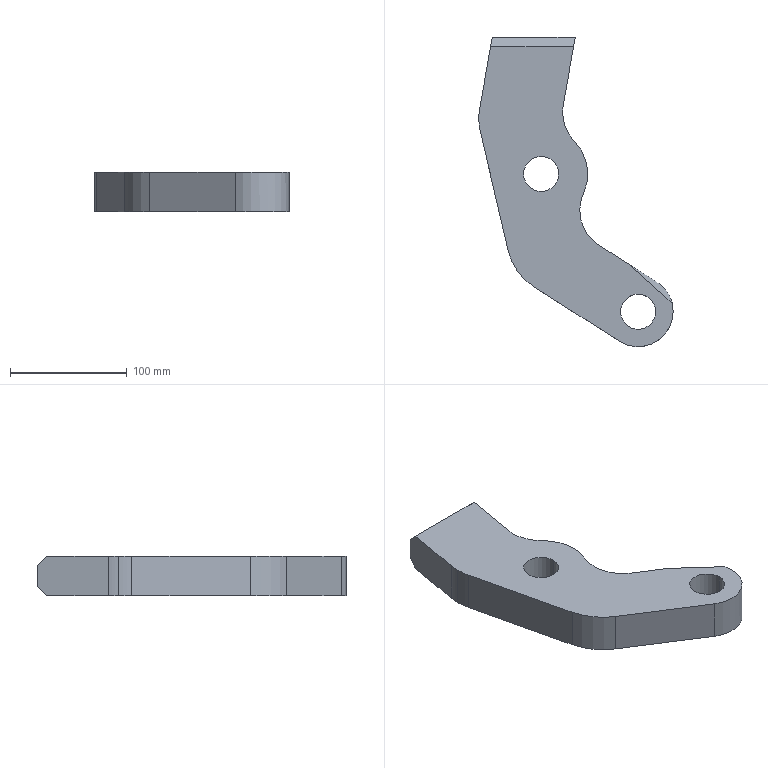Part | SolidWorks | features Fillet 2, ICE 2, Chamfer 1, Extrusion 1 | 1 solid | 24 faces | box 166.468 x 265 x 34 mm | volume 645452 mm3 | cylinder 13 | plane 11 | commonest cylinder face diameters 30 x4 70 x4 100 x3 60 x1 80 x1
STEP:
#1=CARTESIAN_POINT('',(-136.468,165.588,34.));
#2=VERTEX_POINT('',#1);
#3=CARTESIAN_POINT('',(-135.158,154.218,34.));
#4=VERTEX_POINT('',#3);
#5=CARTESIAN_POINT('',(-86.468,165.588,34.));
#6=DIRECTION('',(0.,0.,1.));
#7=DIRECTION('',(1.,0.,0.));
#8=AXIS2_PLACEMENT_3D('',#5,#6,#7);
#9=CIRCLE('',#8,50.);
#10=EDGE_CURVE('',#2,#4,#9,.T.);
#11=ORIENTED_EDGE('',*,*,#10,.F.);
#12=CARTESIAN_POINT('',(-136.468,165.588,0.));
#13=VERTEX_POINT('',#12);
#14=CARTESIAN_POINT('',(-136.468,165.588,34.));
#15=DIRECTION('',(0.,0.,-1.));
#16=VECTOR('',#15,1000.);
#17=LINE('',#14,#16);
#18=EDGE_CURVE('',#2,#13,#17,.T.);
#19=ORIENTED_EDGE('',*,*,#18,.T.);
#20=CARTESIAN_POINT('',(-135.158,154.218,0.));
#21=VERTEX_POINT('',#20);
#22=CARTESIAN_POINT('',(-86.468,165.588,0.));
#23=DIRECTION('',(0.,0.,-1.));
#24=DIRECTION('',(1.,0.,0.));
#25=AXIS2_PLACEMENT_3D('',#22,#23,#24);
#26=CIRCLE('',#25,50.);
#27=EDGE_CURVE('',#21,#13,#26,.T.);
#28=ORIENTED_EDGE('',*,*,#27,.F.);
#29=CARTESIAN_POINT('',(-135.158,154.218,34.));
#30=DIRECTION('',(0.,0.,-1.));
#31=VECTOR('',#30,1000.);
#32=LINE('',#29,#31);
#33=EDGE_CURVE('',#4,#21,#32,.T.);
#34=ORIENTED_EDGE('',*,*,#33,.F.);
#35=EDGE_LOOP('',(#11,#19,#28,#34));
#36=FACE_OUTER_BOUND('',#35,.T.);
#37=CARTESIAN_POINT('',(-86.468,165.588,34.));
#38=DIRECTION('',(0.,0.,-1.));
#39=DIRECTION('',(-1.,0.,0.));
#40=AXIS2_PLACEMENT_3D('',#37,#38,#39);
#41=CYLINDRICAL_SURFACE('',#40,50.);
#42=ADVANCED_FACE('',(#36),#41,.T.);
#43=CARTESIAN_POINT('',(-64.722,170.676,34.));
#44=VERTEX_POINT('',#43);
#45=CARTESIAN_POINT('',(-64.19,176.753,34.));
#46=VERTEX_POINT('',#45);
#47=CARTESIAN_POINT('',(-29.722,170.676,34.));
#48=DIRECTION('',(0.,0.,-1.));
#49=DIRECTION('',(1.,0.,0.));
#50=AXIS2_PLACEMENT_3D('',#47,#48,#49);
#51=CIRCLE('',#50,35.);
#52=EDGE_CURVE('',#44,#46,#51,.T.);
#53=ORIENTED_EDGE('',*,*,#52,.F.);
#54=CARTESIAN_POINT('',(-64.722,170.676,0.));
#55=VERTEX_POINT('',#54);
#56=CARTESIAN_POINT('',(-64.722,170.676,34.));
#57=DIRECTION('',(0.,0.,-1.));
#58=VECTOR('',#57,1000.);
#59=LINE('',#56,#58);
#60=EDGE_CURVE('',#44,#55,#59,.T.);
#61=ORIENTED_EDGE('',*,*,#60,.T.);
#62=CARTESIAN_POINT('',(-64.19,176.753,0.));
#63=VERTEX_POINT('',#62);
#64=CARTESIAN_POINT('',(-29.722,170.676,0.));
#65=DIRECTION('',(0.,0.,1.));
#66=DIRECTION('',(1.,0.,0.));
#67=AXIS2_PLACEMENT_3D('',#64,#65,#66);
#68=CIRCLE('',#67,35.);
#69=EDGE_CURVE('',#63,#55,#68,.T.);
#70=ORIENTED_EDGE('',*,*,#69,.F.);
#71=CARTESIAN_POINT('',(-64.19,176.753,0.));
#72=DIRECTION('',(0.,0.,-1.));
#73=VECTOR('',#72,1000.);
#74=LINE('',#71,#73);
#75=EDGE_CURVE('',#46,#63,#74,.T.);
#76=ORIENTED_EDGE('',*,*,#75,.F.);
#77=EDGE_LOOP('',(#53,#61,#70,#76));
#78=FACE_OUTER_BOUND('',#77,.T.);
#79=CARTESIAN_POINT('',(-29.722,170.676,34.));
#80=DIRECTION('',(0.,0.,-1.));
#81=DIRECTION('',(-1.,0.,0.));
#82=AXIS2_PLACEMENT_3D('',#79,#80,#81);
#83=CYLINDRICAL_SURFACE('',#82,35.);
#84=ADVANCED_FACE('',(#78),#83,.F.);
#85=CARTESIAN_POINT('',(-49.979,86.645,34.));
#86=VERTEX_POINT('',#85);
#87=CARTESIAN_POINT('',(-46.773,101.277,34.));
#88=VERTEX_POINT('',#87);
#89=CARTESIAN_POINT('',(-14.979,86.645,34.));
#90=DIRECTION('',(0.,0.,-1.));
#91=DIRECTION('',(1.,0.,0.));
#92=AXIS2_PLACEMENT_3D('',#89,#90,#91);
#93=CIRCLE('',#92,35.);
#94=EDGE_CURVE('',#86,#88,#93,.T.);
#95=ORIENTED_EDGE('',*,*,#94,.F.);
#96=CARTESIAN_POINT('',(-49.979,86.645,0.));
#97=VERTEX_POINT('',#96);
#98=CARTESIAN_POINT('',(-49.979,86.645,34.));
#99=DIRECTION('',(0.,0.,-1.));
#100=VECTOR('',#99,1000.);
#101=LINE('',#98,#100);
#102=EDGE_CURVE('',#86,#97,#101,.T.);
#103=ORIENTED_EDGE('',*,*,#102,.T.);
#104=CARTESIAN_POINT('',(-46.773,101.277,0.));
#105=VERTEX_POINT('',#104);
#106=CARTESIAN_POINT('',(-14.979,86.645,0.));
#107=DIRECTION('',(0.,0.,1.));
#108=DIRECTION('',(1.,0.,0.));
#109=AXIS2_PLACEMENT_3D('',#106,#107,#108);
#110=CIRCLE('',#109,35.);
#111=EDGE_CURVE('',#105,#97,#110,.T.);
#112=ORIENTED_EDGE('',*,*,#111,.F.);
#113=CARTESIAN_POINT('',(-46.773,101.277,34.));
#114=DIRECTION('',(0.,0.,-1.));
#115=VECTOR('',#114,1000.);
#116=LINE('',#113,#115);
#117=EDGE_CURVE('',#88,#105,#116,.T.);
#118=ORIENTED_EDGE('',*,*,#117,.F.);
#119=EDGE_LOOP('',(#95,#103,#112,#118));
#120=FACE_OUTER_BOUND('',#119,.T.);
#121=CARTESIAN_POINT('',(-14.979,86.645,34.));
#122=DIRECTION('',(0.,0.,-1.));
#123=DIRECTION('',(-1.,0.,0.));
#124=AXIS2_PLACEMENT_3D('',#121,#122,#123);
#125=CYLINDRICAL_SURFACE('',#124,35.);
#126=ADVANCED_FACE('',(#120),#125,.F.);
#127=CARTESIAN_POINT('',(-68.121,118.,34.));
#128=VERTEX_POINT('',#127);
#129=CARTESIAN_POINT('',(-98.121,118.,34.));
#130=VERTEX_POINT('',#129);
#131=CARTESIAN_POINT('',(-83.121,118.,34.));
#132=DIRECTION('',(0.,0.,-1.));
#133=DIRECTION('',(-1.,0.,0.));
#134=AXIS2_PLACEMENT_3D('',#131,#132,#133);
#135=CIRCLE('',#134,15.);
#136=EDGE_CURVE('',#128,#130,#135,.T.);
#137=ORIENTED_EDGE('',*,*,#136,.F.);
#138=CARTESIAN_POINT('',(-68.121,118.,0.));
#139=VERTEX_POINT('',#138);
#140=CARTESIAN_POINT('',(-68.121,118.,34.));
#141=DIRECTION('',(0.,0.,-1.));
#142=VECTOR('',#141,1000.);
#143=LINE('',#140,#142);
#144=EDGE_CURVE('',#128,#139,#143,.T.);
#145=ORIENTED_EDGE('',*,*,#144,.T.);
#146=CARTESIAN_POINT('',(-98.121,118.,0.));
#147=VERTEX_POINT('',#146);
#148=CARTESIAN_POINT('',(-83.121,118.,0.));
#149=DIRECTION('',(0.,0.,-1.));
#150=DIRECTION('',(-1.,0.,0.));
#151=AXIS2_PLACEMENT_3D('',#148,#149,#150);
#152=CIRCLE('',#151,15.);
#153=EDGE_CURVE('',#139,#147,#152,.T.);
#154=ORIENTED_EDGE('',*,*,#153,.T.);
#155=CARTESIAN_POINT('',(-98.121,118.,34.));
#156=DIRECTION('',(0.,0.,-1.));
#157=VECTOR('',#156,1000.);
#158=LINE('',#155,#157);
#159=EDGE_CURVE('',#130,#147,#158,.T.);
#160=ORIENTED_EDGE('',*,*,#159,.F.);
#161=EDGE_LOOP('',(#137,#145,#154,#160));
#162=FACE_OUTER_BOUND('',#161,.T.);
#163=CARTESIAN_POINT('',(-83.121,118.,34.));
#164=DIRECTION('',(0.,0.,-1.));
#165=DIRECTION('',(-1.,0.,0.));
#166=AXIS2_PLACEMENT_3D('',#163,#164,#165);
#167=CYLINDRICAL_SURFACE('',#166,15.);
#168=ADVANCED_FACE('',(#162),#167,.F.);
#169=CARTESIAN_POINT('',(14.992,0.,34.));
#170=VERTEX_POINT('',#169);
#171=CARTESIAN_POINT('',(-15.008,0.,34.));
#172=VERTEX_POINT('',#171);
#173=CARTESIAN_POINT('',(-0.008419,0.,34.));
#174=DIRECTION('',(0.,0.,-1.));
#175=DIRECTION('',(-1.,0.,0.));
#176=AXIS2_PLACEMENT_3D('',#173,#174,#175);
#177=CIRCLE('',#176,15.);
#178=EDGE_CURVE('',#170,#172,#177,.T.);
#179=ORIENTED_EDGE('',*,*,#178,.F.);
#180=CARTESIAN_POINT('',(14.992,0.,0.));
#181=VERTEX_POINT('',#180);
#182=CARTESIAN_POINT('',(14.992,0.,34.));
#183=DIRECTION('',(0.,0.,-1.));
#184=VECTOR('',#183,1000.);
#185=LINE('',#182,#184);
#186=EDGE_CURVE('',#170,#181,#185,.T.);
#187=ORIENTED_EDGE('',*,*,#186,.T.);
#188=CARTESIAN_POINT('',(-15.008,0.,0.));
#189=VERTEX_POINT('',#188);
#190=CARTESIAN_POINT('',(-0.008419,0.,0.));
#191=DIRECTION('',(0.,0.,-1.));
#192=DIRECTION('',(-1.,0.,0.));
#193=AXIS2_PLACEMENT_3D('',#190,#191,#192);
#194=CIRCLE('',#193,15.);
#195=EDGE_CURVE('',#181,#189,#194,.T.);
#196=ORIENTED_EDGE('',*,*,#195,.T.);
#197=CARTESIAN_POINT('',(-15.008,0.,34.));
#198=DIRECTION('',(0.,0.,-1.));
#199=VECTOR('',#198,1000.);
#200=LINE('',#197,#199);
#201=EDGE_CURVE('',#172,#189,#200,.T.);
#202=ORIENTED_EDGE('',*,*,#201,.F.);
#203=EDGE_LOOP('',(#179,#187,#196,#202));
#204=FACE_OUTER_BOUND('',#203,.T.);
#205=CARTESIAN_POINT('',(-0.008419,0.,34.));
#206=DIRECTION('',(0.,0.,-1.));
#207=DIRECTION('',(-1.,0.,0.));
#208=AXIS2_PLACEMENT_3D('',#205,#206,#207);
#209=CYLINDRICAL_SURFACE('',#208,15.);
#210=ADVANCED_FACE('',(#204),#209,.F.);
#211=CARTESIAN_POINT('',(-55.331,227.,34.));
#212=VERTEX_POINT('',#211);
#213=CARTESIAN_POINT('',(-53.92,235.,34.));
#214=DIRECTION('',(0.1736,0.9848,0.));
#215=VECTOR('',#214,1000.);
#216=LINE('',#213,#215);
#217=EDGE_CURVE('',#46,#212,#216,.T.);
#218=ORIENTED_EDGE('',*,*,#217,.F.);
#219=ORIENTED_EDGE('',*,*,#75,.T.);
#220=CARTESIAN_POINT('',(-55.331,227.,0.));
#221=VERTEX_POINT('',#220);
#222=CARTESIAN_POINT('',(-53.92,235.,0.));
#223=DIRECTION('',(0.1736,0.9848,0.));
#224=VECTOR('',#223,1000.);
#225=LINE('',#222,#224);
#226=EDGE_CURVE('',#63,#221,#225,.T.);
#227=ORIENTED_EDGE('',*,*,#226,.T.);
#228=CARTESIAN_POINT('',(-53.92,235.,8.));
#229=VERTEX_POINT('',#228);
#230=CARTESIAN_POINT('',(-55.008,228.829,1.829));
#231=DIRECTION('',(0.1237,0.7017,0.7017));
#232=VECTOR('',#231,1000.);
#233=LINE('',#230,#232);
#234=EDGE_CURVE('',#221,#229,#233,.T.);
#235=ORIENTED_EDGE('',*,*,#234,.T.);
#236=CARTESIAN_POINT('',(-53.92,235.,26.));
#237=VERTEX_POINT('',#236);
#238=CARTESIAN_POINT('',(-53.92,235.,34.));
#239=DIRECTION('',(0.,0.,-1.));
#240=VECTOR('',#239,1000.);
#241=LINE('',#238,#240);
#242=EDGE_CURVE('',#237,#229,#241,.T.);
#243=ORIENTED_EDGE('',*,*,#242,.F.);
#244=CARTESIAN_POINT('',(-55.756,224.588,36.412));
#245=DIRECTION('',(-0.1237,-0.7017,0.7017));
#246=VECTOR('',#245,1000.);
#247=LINE('',#244,#246);
#248=EDGE_CURVE('',#237,#212,#247,.T.);
#249=ORIENTED_EDGE('',*,*,#248,.T.);
#250=EDGE_LOOP('',(#218,#219,#227,#235,#243,#249));
#251=FACE_OUTER_BOUND('',#250,.T.);
#252=CARTESIAN_POINT('',(-53.92,235.,34.));
#253=DIRECTION('',(-0.9848,0.1736,0.));
#254=DIRECTION('',(-0.1736,-0.9848,0.));
#255=AXIS2_PLACEMENT_3D('',#252,#253,#254);
#256=PLANE('',#255);
#257=ADVANCED_FACE('',(#251),#256,.F.);
#258=ORIENTED_EDGE('',*,*,#242,.T.);
#259=CARTESIAN_POINT('',(-125.,235.,8.));
#260=VERTEX_POINT('',#259);
#261=CARTESIAN_POINT('',(-125.,235.,8.));
#262=DIRECTION('',(-1.,0.,0.));
#263=VECTOR('',#262,1000.);
#264=LINE('',#261,#263);
#265=EDGE_CURVE('',#229,#260,#264,.T.);
#266=ORIENTED_EDGE('',*,*,#265,.T.);
#267=CARTESIAN_POINT('',(-125.,235.,26.));
#268=VERTEX_POINT('',#267);
#269=CARTESIAN_POINT('',(-125.,235.,34.));
#270=DIRECTION('',(0.,0.,-1.));
#271=VECTOR('',#270,1000.);
#272=LINE('',#269,#271);
#273=EDGE_CURVE('',#268,#260,#272,.T.);
#274=ORIENTED_EDGE('',*,*,#273,.F.);
#275=CARTESIAN_POINT('',(-53.92,235.,26.));
#276=DIRECTION('',(1.,0.,0.));
#277=VECTOR('',#276,1000.);
#278=LINE('',#275,#277);
#279=EDGE_CURVE('',#268,#237,#278,.T.);
#280=ORIENTED_EDGE('',*,*,#279,.T.);
#281=EDGE_LOOP('',(#258,#266,#274,#280));
#282=FACE_OUTER_BOUND('',#281,.T.);
#283=CARTESIAN_POINT('',(-125.,235.,34.));
#284=DIRECTION('',(0.,-1.,0.));
#285=DIRECTION('',(0.,0.,-1.));
#286=AXIS2_PLACEMENT_3D('',#283,#284,#285);
#287=PLANE('',#286);
#288=ADVANCED_FACE('',(#282),#287,.F.);
#289=CARTESIAN_POINT('',(-126.411,227.,0.));
#290=VERTEX_POINT('',#289);
#291=CARTESIAN_POINT('',(-135.708,174.271,0.));
#292=VERTEX_POINT('',#291);
#293=CARTESIAN_POINT('',(-125.,235.,0.));
#294=DIRECTION('',(-0.1736,-0.9848,0.));
#295=VECTOR('',#294,1000.);
#296=LINE('',#293,#295);
#297=EDGE_CURVE('',#290,#292,#296,.T.);
#298=ORIENTED_EDGE('',*,*,#297,.T.);
#299=CARTESIAN_POINT('',(-135.708,174.271,34.));
#300=VERTEX_POINT('',#299);
#301=CARTESIAN_POINT('',(-135.708,174.271,34.));
#302=DIRECTION('',(0.,0.,1.));
#303=VECTOR('',#302,1000.);
#304=LINE('',#301,#303);
#305=EDGE_CURVE('',#292,#300,#304,.T.);
#306=ORIENTED_EDGE('',*,*,#305,.T.);
#307=CARTESIAN_POINT('',(-126.411,227.,34.));
#308=VERTEX_POINT('',#307);
#309=CARTESIAN_POINT('',(-125.,235.,34.));
#310=DIRECTION('',(-0.1736,-0.9848,0.));
#311=VECTOR('',#310,1000.);
#312=LINE('',#309,#311);
#313=EDGE_CURVE('',#308,#300,#312,.T.);
#314=ORIENTED_EDGE('',*,*,#313,.F.);
#315=CARTESIAN_POINT('',(-125.748,230.759,30.241));
#316=DIRECTION('',(0.1237,0.7017,-0.7017));
#317=VECTOR('',#316,1000.);
#318=LINE('',#315,#317);
#319=EDGE_CURVE('',#308,#268,#318,.T.);
#320=ORIENTED_EDGE('',*,*,#319,.T.);
#321=ORIENTED_EDGE('',*,*,#273,.T.);
#322=CARTESIAN_POINT('',(-125.,235.,8.));
#323=DIRECTION('',(-0.1237,-0.7017,-0.7017));
#324=VECTOR('',#323,1000.);
#325=LINE('',#322,#324);
#326=EDGE_CURVE('',#260,#290,#325,.T.);
#327=ORIENTED_EDGE('',*,*,#326,.T.);
#328=EDGE_LOOP('',(#298,#306,#314,#320,#321,#327));
#329=FACE_OUTER_BOUND('',#328,.T.);
#330=CARTESIAN_POINT('',(-125.,235.,34.));
#331=DIRECTION('',(0.9848,-0.1736,0.));
#332=DIRECTION('',(0.1736,0.9848,0.));
#333=AXIS2_PLACEMENT_3D('',#330,#331,#332);
#334=PLANE('',#333);
#335=ADVANCED_FACE('',(#329),#334,.F.);
#336=CARTESIAN_POINT('',(-111.36,52.316,0.));
#337=VERTEX_POINT('',#336);
#338=CARTESIAN_POINT('',(-137.486,164.188,0.));
#339=DIRECTION('',(0.2274,-0.9738,0.));
#340=VECTOR('',#339,1000.);
#341=LINE('',#338,#340);
#342=EDGE_CURVE('',#21,#337,#341,.T.);
#343=ORIENTED_EDGE('',*,*,#342,.T.);
#344=CARTESIAN_POINT('',(-111.36,52.316,34.));
#345=VERTEX_POINT('',#344);
#346=CARTESIAN_POINT('',(-111.36,52.316,34.));
#347=DIRECTION('',(0.,0.,1.));
#348=VECTOR('',#347,1000.);
#349=LINE('',#346,#348);
#350=EDGE_CURVE('',#337,#345,#349,.T.);
#351=ORIENTED_EDGE('',*,*,#350,.T.);
#352=CARTESIAN_POINT('',(-137.486,164.188,34.));
#353=DIRECTION('',(0.2274,-0.9738,0.));
#354=VECTOR('',#353,1000.);
#355=LINE('',#352,#354);
#356=EDGE_CURVE('',#4,#345,#355,.T.);
#357=ORIENTED_EDGE('',*,*,#356,.F.);
#358=ORIENTED_EDGE('',*,*,#33,.T.);
#359=EDGE_LOOP('',(#343,#351,#357,#358));
#360=FACE_OUTER_BOUND('',#359,.T.);
#361=CARTESIAN_POINT('',(-137.486,164.188,34.));
#362=DIRECTION('',(0.9738,0.2274,0.));
#363=DIRECTION('',(-0.2274,0.9738,0.));
#364=AXIS2_PLACEMENT_3D('',#361,#362,#363);
#365=PLANE('',#364);
#366=ADVANCED_FACE('',(#360),#365,.F.);
#367=CARTESIAN_POINT('',(-89.555,21.529,34.));
#368=VERTEX_POINT('',#367);
#369=CARTESIAN_POINT('',(-16.131,-25.294,34.));
#370=VERTEX_POINT('',#369);
#371=CARTESIAN_POINT('',(-106.728,32.481,34.));
#372=DIRECTION('',(0.8431,-0.5377,0.));
#373=VECTOR('',#372,1000.);
#374=LINE('',#371,#373);
#375=EDGE_CURVE('',#368,#370,#374,.T.);
#376=ORIENTED_EDGE('',*,*,#375,.F.);
#377=CARTESIAN_POINT('',(-89.555,21.529,0.));
#378=VERTEX_POINT('',#377);
#379=CARTESIAN_POINT('',(-89.555,21.529,34.));
#380=DIRECTION('',(0.,0.,-1.));
#381=VECTOR('',#380,1000.);
#382=LINE('',#379,#381);
#383=EDGE_CURVE('',#368,#378,#382,.T.);
#384=ORIENTED_EDGE('',*,*,#383,.T.);
#385=CARTESIAN_POINT('',(-16.131,-25.294,0.));
#386=VERTEX_POINT('',#385);
#387=CARTESIAN_POINT('',(-106.728,32.481,0.));
#388=DIRECTION('',(0.8431,-0.5377,0.));
#389=VECTOR('',#388,1000.);
#390=LINE('',#387,#389);
#391=EDGE_CURVE('',#378,#386,#390,.T.);
#392=ORIENTED_EDGE('',*,*,#391,.T.);
#393=CARTESIAN_POINT('',(-16.131,-25.294,34.));
#394=DIRECTION('',(0.,0.,-1.));
#395=VECTOR('',#394,1000.);
#396=LINE('',#393,#395);
#397=EDGE_CURVE('',#370,#386,#396,.T.);
#398=ORIENTED_EDGE('',*,*,#397,.F.);
#399=EDGE_LOOP('',(#376,#384,#392,#398));
#400=FACE_OUTER_BOUND('',#399,.T.);
#401=CARTESIAN_POINT('',(-106.728,32.481,34.));
#402=DIRECTION('',(0.5377,0.8431,0.));
#403=DIRECTION('',(-0.8431,0.5377,0.));
#404=AXIS2_PLACEMENT_3D('',#401,#402,#403);
#405=PLANE('',#404);
#406=ADVANCED_FACE('',(#400),#405,.F.);
#407=CARTESIAN_POINT('',(16.131,25.294,22.982));
#408=VERTEX_POINT('',#407);
#409=CARTESIAN_POINT('',(29.052,7.482,34.));
#410=VERTEX_POINT('',#409);
#411=CARTESIAN_POINT('',(16.131,25.294,22.982));
#412=CARTESIAN_POINT('',(22.616,21.158,19.943));
#413=CARTESIAN_POINT('',(27.133,14.932,23.795));
#414=CARTESIAN_POINT('',(29.052,7.482,34.));
#415=(BOUNDED_CURVE()B_SPLINE_CURVE(3,(#411,#412,#413,#414),.UNSPECIFIED.,.F.,.F.)B_SPLINE_CURVE_WITH_KNOTS((4,4),(6.118,6.869),.UNSPECIFIED.)CURVE()GEOMETRIC_REPRESENTATION_ITEM()RATIONAL_B_SPLINE_CURVE((1.,0.9535,0.9535,1.))REPRESENTATION_ITEM(''));
#416=EDGE_CURVE('',#408,#410,#415,.T.);
#417=ORIENTED_EDGE('',*,*,#416,.T.);
#418=CARTESIAN_POINT('',(0.,0.,34.));
#419=DIRECTION('',(0.,0.,1.));
#420=DIRECTION('',(1.,0.,0.));
#421=AXIS2_PLACEMENT_3D('',#418,#419,#420);
#422=CIRCLE('',#421,30.);
#423=EDGE_CURVE('',#370,#410,#422,.T.);
#424=ORIENTED_EDGE('',*,*,#423,.F.);
#425=ORIENTED_EDGE('',*,*,#397,.T.);
#426=CARTESIAN_POINT('',(16.131,25.294,0.));
#427=VERTEX_POINT('',#426);
#428=CARTESIAN_POINT('',(0.,0.,0.));
#429=DIRECTION('',(0.,0.,1.));
#430=DIRECTION('',(1.,0.,0.));
#431=AXIS2_PLACEMENT_3D('',#428,#429,#430);
#432=CIRCLE('',#431,30.);
#433=EDGE_CURVE('',#386,#427,#432,.T.);
#434=ORIENTED_EDGE('',*,*,#433,.T.);
#435=CARTESIAN_POINT('',(16.131,25.294,34.));
#436=DIRECTION('',(0.,0.,-1.));
#437=VECTOR('',#436,1000.);
#438=LINE('',#435,#437);
#439=EDGE_CURVE('',#408,#427,#438,.T.);
#440=ORIENTED_EDGE('',*,*,#439,.F.);
#441=EDGE_LOOP('',(#417,#424,#425,#434,#440));
#442=FACE_OUTER_BOUND('',#441,.T.);
#443=CARTESIAN_POINT('',(0.,0.,34.));
#444=DIRECTION('',(0.,0.,-1.));
#445=DIRECTION('',(-1.,0.,0.));
#446=AXIS2_PLACEMENT_3D('',#443,#444,#445);
#447=CYLINDRICAL_SURFACE('',#446,30.);
#448=ADVANCED_FACE('',(#442),#447,.T.);
#449=CARTESIAN_POINT('',(-7.386,40.291,34.));
#450=VERTEX_POINT('',#449);
#451=CARTESIAN_POINT('',(-33.798,57.134,34.));
#452=VERTEX_POINT('',#451);
#453=CARTESIAN_POINT('',(-69.988,80.214,34.));
#454=DIRECTION('',(-0.8431,0.5377,0.));
#455=VECTOR('',#454,1000.);
#456=LINE('',#453,#455);
#457=EDGE_CURVE('',#450,#452,#456,.T.);
#458=ORIENTED_EDGE('',*,*,#457,.F.);
#459=CARTESIAN_POINT('',(-61.538,74.825,59.371));
#460=DIRECTION('',(0.7842,-0.5001,-0.3674));
#461=VECTOR('',#460,1000.);
#462=LINE('',#459,#461);
#463=EDGE_CURVE('',#450,#408,#462,.T.);
#464=ORIENTED_EDGE('',*,*,#463,.T.);
#465=ORIENTED_EDGE('',*,*,#439,.T.);
#466=CARTESIAN_POINT('',(-33.798,57.134,0.));
#467=VERTEX_POINT('',#466);
#468=CARTESIAN_POINT('',(-69.988,80.214,0.));
#469=DIRECTION('',(-0.8431,0.5377,0.));
#470=VECTOR('',#469,1000.);
#471=LINE('',#468,#470);
#472=EDGE_CURVE('',#427,#467,#471,.T.);
#473=ORIENTED_EDGE('',*,*,#472,.T.);
#474=CARTESIAN_POINT('',(-33.798,57.134,34.));
#475=DIRECTION('',(0.,0.,1.));
#476=VECTOR('',#475,1000.);
#477=LINE('',#474,#476);
#478=EDGE_CURVE('',#467,#452,#477,.T.);
#479=ORIENTED_EDGE('',*,*,#478,.T.);
#480=EDGE_LOOP('',(#458,#464,#465,#473,#479));
#481=FACE_OUTER_BOUND('',#480,.T.);
#482=CARTESIAN_POINT('',(-69.988,80.214,34.));
#483=DIRECTION('',(-0.5377,-0.8431,0.));
#484=DIRECTION('',(0.8431,-0.5377,0.));
#485=AXIS2_PLACEMENT_3D('',#482,#483,#484);
#486=PLANE('',#485);
#487=ADVANCED_FACE('',(#481),#486,.F.);
#488=CARTESIAN_POINT('',(-54.636,146.094,34.));
#489=VERTEX_POINT('',#488);
#490=CARTESIAN_POINT('',(-83.11,118.,34.));
#491=DIRECTION('',(0.,0.,1.));
#492=DIRECTION('',(1.,0.,0.));
#493=AXIS2_PLACEMENT_3D('',#490,#491,#492);
#494=CIRCLE('',#493,40.);
#495=EDGE_CURVE('',#88,#489,#494,.T.);
#496=ORIENTED_EDGE('',*,*,#495,.F.);
#497=ORIENTED_EDGE('',*,*,#117,.T.);
#498=CARTESIAN_POINT('',(-54.636,146.094,0.));
#499=VERTEX_POINT('',#498);
#500=CARTESIAN_POINT('',(-83.11,118.,0.));
#501=DIRECTION('',(0.,0.,1.));
#502=DIRECTION('',(1.,0.,0.));
#503=AXIS2_PLACEMENT_3D('',#500,#501,#502);
#504=CIRCLE('',#503,40.);
#505=EDGE_CURVE('',#105,#499,#504,.T.);
#506=ORIENTED_EDGE('',*,*,#505,.T.);
#507=CARTESIAN_POINT('',(-54.636,146.094,34.));
#508=DIRECTION('',(0.,0.,1.));
#509=VECTOR('',#508,1000.);
#510=LINE('',#507,#509);
#511=EDGE_CURVE('',#499,#489,#510,.T.);
#512=ORIENTED_EDGE('',*,*,#511,.T.);
#513=EDGE_LOOP('',(#496,#497,#506,#512));
#514=FACE_OUTER_BOUND('',#513,.T.);
#515=CARTESIAN_POINT('',(-83.11,118.,34.));
#516=DIRECTION('',(0.,0.,-1.));
#517=DIRECTION('',(-1.,0.,0.));
#518=AXIS2_PLACEMENT_3D('',#515,#516,#517);
#519=CYLINDRICAL_SURFACE('',#518,40.);
#520=ADVANCED_FACE('',(#514),#519,.T.);
#521=CARTESIAN_POINT('',(-175.495,191.658,34.));
#522=DIRECTION('',(0.7431,-0.6691,0.));
#523=VECTOR('',#522,1000.);
#524=LINE('',#521,#523);
#525=EDGE_CURVE('',#450,#410,#524,.T.);
#526=ORIENTED_EDGE('',*,*,#525,.F.);
#527=ORIENTED_EDGE('',*,*,#457,.T.);
#528=CARTESIAN_POINT('',(-14.979,86.645,34.));
#529=DIRECTION('',(0.,0.,-1.));
#530=DIRECTION('',(1.,0.,0.));
#531=AXIS2_PLACEMENT_3D('',#528,#529,#530);
#532=CIRCLE('',#531,35.);
#533=EDGE_CURVE('',#452,#86,#532,.T.);
#534=ORIENTED_EDGE('',*,*,#533,.T.);
#535=ORIENTED_EDGE('',*,*,#94,.T.);
#536=ORIENTED_EDGE('',*,*,#495,.T.);
#537=CARTESIAN_POINT('',(-29.722,170.676,34.));
#538=DIRECTION('',(0.,0.,-1.));
#539=DIRECTION('',(1.,0.,0.));
#540=AXIS2_PLACEMENT_3D('',#537,#538,#539);
#541=CIRCLE('',#540,35.);
#542=EDGE_CURVE('',#489,#44,#541,.T.);
#543=ORIENTED_EDGE('',*,*,#542,.T.);
#544=ORIENTED_EDGE('',*,*,#52,.T.);
#545=ORIENTED_EDGE('',*,*,#217,.T.);
#546=CARTESIAN_POINT('',(-125.,227.,34.));
#547=DIRECTION('',(-1.,0.,0.));
#548=VECTOR('',#547,1000.);
#549=LINE('',#546,#548);
#550=EDGE_CURVE('',#212,#308,#549,.T.);
#551=ORIENTED_EDGE('',*,*,#550,.T.);
#552=ORIENTED_EDGE('',*,*,#313,.T.);
#553=CARTESIAN_POINT('',(-86.468,165.588,34.));
#554=DIRECTION('',(0.,0.,1.));
#555=DIRECTION('',(1.,0.,0.));
#556=AXIS2_PLACEMENT_3D('',#553,#554,#555);
#557=CIRCLE('',#556,50.);
#558=EDGE_CURVE('',#300,#2,#557,.T.);
#559=ORIENTED_EDGE('',*,*,#558,.T.);
#560=ORIENTED_EDGE('',*,*,#10,.T.);
#561=ORIENTED_EDGE('',*,*,#356,.T.);
#562=CARTESIAN_POINT('',(-62.67,63.686,34.));
#563=DIRECTION('',(0.,0.,1.));
#564=DIRECTION('',(1.,0.,0.));
#565=AXIS2_PLACEMENT_3D('',#562,#563,#564);
#566=CIRCLE('',#565,50.);
#567=EDGE_CURVE('',#345,#368,#566,.T.);
#568=ORIENTED_EDGE('',*,*,#567,.T.);
#569=ORIENTED_EDGE('',*,*,#375,.T.);
#570=ORIENTED_EDGE('',*,*,#423,.T.);
#571=EDGE_LOOP('',(#526,#527,#534,#535,#536,#543,#544,#545,#551,#552,#559,#560,#561,#568,#569,#570));
#572=FACE_OUTER_BOUND('',#571,.T.);
#573=CARTESIAN_POINT('',(-83.121,118.,34.));
#574=DIRECTION('',(0.,0.,-1.));
#575=DIRECTION('',(-1.,0.,0.));
#576=AXIS2_PLACEMENT_3D('',#573,#574,#575);
#577=CIRCLE('',#576,15.);
#578=EDGE_CURVE('',#130,#128,#577,.T.);
#579=ORIENTED_EDGE('',*,*,#578,.T.);
#580=ORIENTED_EDGE('',*,*,#136,.T.);
#581=EDGE_LOOP('',(#579,#580));
#582=FACE_BOUND('',#581,.T.);
#583=CARTESIAN_POINT('',(-0.008419,0.,34.));
#584=DIRECTION('',(0.,0.,-1.));
#585=DIRECTION('',(-1.,0.,0.));
#586=AXIS2_PLACEMENT_3D('',#583,#584,#585);
#587=CIRCLE('',#586,15.);
#588=EDGE_CURVE('',#172,#170,#587,.T.);
#589=ORIENTED_EDGE('',*,*,#588,.T.);
#590=ORIENTED_EDGE('',*,*,#178,.T.);
#591=EDGE_LOOP('',(#589,#590));
#592=FACE_BOUND('',#591,.T.);
#593=CARTESIAN_POINT('',(-83.11,118.,34.));
#594=DIRECTION('',(0.,0.,1.));
#595=DIRECTION('',(1.,0.,0.));
#596=AXIS2_PLACEMENT_3D('',#593,#594,#595);
#597=PLANE('',#596);
#598=ADVANCED_FACE('',(#572,#582,#592),#597,.T.);
#599=CARTESIAN_POINT('',(-83.121,118.,0.));
#600=DIRECTION('',(0.,0.,-1.));
#601=DIRECTION('',(-1.,0.,0.));
#602=AXIS2_PLACEMENT_3D('',#599,#600,#601);
#603=CIRCLE('',#602,15.);
#604=EDGE_CURVE('',#147,#139,#603,.T.);
#605=ORIENTED_EDGE('',*,*,#604,.F.);
#606=ORIENTED_EDGE('',*,*,#153,.F.);
#607=EDGE_LOOP('',(#605,#606));
#608=FACE_BOUND('',#607,.T.);
#609=CARTESIAN_POINT('',(-0.008419,0.,0.));
#610=DIRECTION('',(0.,0.,-1.));
#611=DIRECTION('',(-1.,0.,0.));
#612=AXIS2_PLACEMENT_3D('',#609,#610,#611);
#613=CIRCLE('',#612,15.);
#614=EDGE_CURVE('',#189,#181,#613,.T.);
#615=ORIENTED_EDGE('',*,*,#614,.F.);
#616=ORIENTED_EDGE('',*,*,#195,.F.);
#617=EDGE_LOOP('',(#615,#616));
#618=FACE_BOUND('',#617,.T.);
#619=ORIENTED_EDGE('',*,*,#391,.F.);
#620=CARTESIAN_POINT('',(-62.67,63.686,0.));
#621=DIRECTION('',(0.,0.,-1.));
#622=DIRECTION('',(1.,0.,0.));
#623=AXIS2_PLACEMENT_3D('',#620,#621,#622);
#624=CIRCLE('',#623,50.);
#625=EDGE_CURVE('',#378,#337,#624,.T.);
#626=ORIENTED_EDGE('',*,*,#625,.T.);
#627=ORIENTED_EDGE('',*,*,#342,.F.);
#628=ORIENTED_EDGE('',*,*,#27,.T.);
#629=CARTESIAN_POINT('',(-86.468,165.588,0.));
#630=DIRECTION('',(0.,0.,-1.));
#631=DIRECTION('',(1.,0.,0.));
#632=AXIS2_PLACEMENT_3D('',#629,#630,#631);
#633=CIRCLE('',#632,50.);
#634=EDGE_CURVE('',#13,#292,#633,.T.);
#635=ORIENTED_EDGE('',*,*,#634,.T.);
#636=ORIENTED_EDGE('',*,*,#297,.F.);
#637=CARTESIAN_POINT('',(-83.11,227.,0.));
#638=DIRECTION('',(1.,0.,0.));
#639=VECTOR('',#638,1000.);
#640=LINE('',#637,#639);
#641=EDGE_CURVE('',#290,#221,#640,.T.);
#642=ORIENTED_EDGE('',*,*,#641,.T.);
#643=ORIENTED_EDGE('',*,*,#226,.F.);
#644=ORIENTED_EDGE('',*,*,#69,.T.);
#645=CARTESIAN_POINT('',(-29.722,170.676,0.));
#646=DIRECTION('',(0.,0.,1.));
#647=DIRECTION('',(1.,0.,0.));
#648=AXIS2_PLACEMENT_3D('',#645,#646,#647);
#649=CIRCLE('',#648,35.);
#650=EDGE_CURVE('',#55,#499,#649,.T.);
#651=ORIENTED_EDGE('',*,*,#650,.T.);
#652=ORIENTED_EDGE('',*,*,#505,.F.);
#653=ORIENTED_EDGE('',*,*,#111,.T.);
#654=CARTESIAN_POINT('',(-14.979,86.645,0.));
#655=DIRECTION('',(0.,0.,1.));
#656=DIRECTION('',(1.,0.,0.));
#657=AXIS2_PLACEMENT_3D('',#654,#655,#656);
#658=CIRCLE('',#657,35.);
#659=EDGE_CURVE('',#97,#467,#658,.T.);
#660=ORIENTED_EDGE('',*,*,#659,.T.);
#661=ORIENTED_EDGE('',*,*,#472,.F.);
#662=ORIENTED_EDGE('',*,*,#433,.F.);
#663=EDGE_LOOP('',(#619,#626,#627,#628,#635,#636,#642,#643,#644,#651,#652,#653,#660,#661,#662));
#664=FACE_OUTER_BOUND('',#663,.T.);
#665=CARTESIAN_POINT('',(-83.11,118.,0.));
#666=DIRECTION('',(0.,0.,1.));
#667=DIRECTION('',(1.,0.,0.));
#668=AXIS2_PLACEMENT_3D('',#665,#666,#667);
#669=PLANE('',#668);
#670=ADVANCED_FACE('',(#608,#618,#664),#669,.F.);
#671=ORIENTED_EDGE('',*,*,#234,.F.);
#672=ORIENTED_EDGE('',*,*,#641,.F.);
#673=ORIENTED_EDGE('',*,*,#326,.F.);
#674=ORIENTED_EDGE('',*,*,#265,.F.);
#675=EDGE_LOOP('',(#671,#672,#673,#674));
#676=FACE_OUTER_BOUND('',#675,.T.);
#677=CARTESIAN_POINT('',(-125.,235.,8.));
#678=DIRECTION('',(0.,-0.7071,0.7071));
#679=DIRECTION('',(-1.,0.,0.));
#680=AXIS2_PLACEMENT_3D('',#677,#678,#679);
#681=PLANE('',#680);
#682=ADVANCED_FACE('',(#676),#681,.F.);
#683=ORIENTED_EDGE('',*,*,#248,.F.);
#684=ORIENTED_EDGE('',*,*,#279,.F.);
#685=ORIENTED_EDGE('',*,*,#319,.F.);
#686=ORIENTED_EDGE('',*,*,#550,.F.);
#687=EDGE_LOOP('',(#683,#684,#685,#686));
#688=FACE_OUTER_BOUND('',#687,.T.);
#689=CARTESIAN_POINT('',(-83.11,227.,34.));
#690=DIRECTION('',(0.,0.7071,0.7071));
#691=DIRECTION('',(1.,0.,0.));
#692=AXIS2_PLACEMENT_3D('',#689,#690,#691);
#693=PLANE('',#692);
#694=ADVANCED_FACE('',(#688),#693,.T.);
#695=ORIENTED_EDGE('',*,*,#186,.F.);
#696=ORIENTED_EDGE('',*,*,#588,.F.);
#697=ORIENTED_EDGE('',*,*,#201,.T.);
#698=ORIENTED_EDGE('',*,*,#614,.T.);
#699=EDGE_LOOP('',(#695,#696,#697,#698));
#700=FACE_OUTER_BOUND('',#699,.T.);
#701=CARTESIAN_POINT('',(-0.008419,0.,34.));
#702=DIRECTION('',(0.,0.,-1.));
#703=DIRECTION('',(-1.,0.,0.));
#704=AXIS2_PLACEMENT_3D('',#701,#702,#703);
#705=CYLINDRICAL_SURFACE('',#704,15.);
#706=ADVANCED_FACE('',(#700),#705,.F.);
#707=ORIENTED_EDGE('',*,*,#144,.F.);
#708=ORIENTED_EDGE('',*,*,#578,.F.);
#709=ORIENTED_EDGE('',*,*,#159,.T.);
#710=ORIENTED_EDGE('',*,*,#604,.T.);
#711=EDGE_LOOP('',(#707,#708,#709,#710));
#712=FACE_OUTER_BOUND('',#711,.T.);
#713=CARTESIAN_POINT('',(-83.121,118.,34.));
#714=DIRECTION('',(0.,0.,-1.));
#715=DIRECTION('',(-1.,0.,0.));
#716=AXIS2_PLACEMENT_3D('',#713,#714,#715);
#717=CYLINDRICAL_SURFACE('',#716,15.);
#718=ADVANCED_FACE('',(#712),#717,.F.);
#719=ORIENTED_EDGE('',*,*,#102,.F.);
#720=ORIENTED_EDGE('',*,*,#533,.F.);
#721=ORIENTED_EDGE('',*,*,#478,.F.);
#722=ORIENTED_EDGE('',*,*,#659,.F.);
#723=EDGE_LOOP('',(#719,#720,#721,#722));
#724=FACE_OUTER_BOUND('',#723,.T.);
#725=CARTESIAN_POINT('',(-14.979,86.645,34.));
#726=DIRECTION('',(0.,0.,-1.));
#727=DIRECTION('',(-1.,0.,0.));
#728=AXIS2_PLACEMENT_3D('',#725,#726,#727);
#729=CYLINDRICAL_SURFACE('',#728,35.);
#730=ADVANCED_FACE('',(#724),#729,.F.);
#731=ORIENTED_EDGE('',*,*,#60,.F.);
#732=ORIENTED_EDGE('',*,*,#542,.F.);
#733=ORIENTED_EDGE('',*,*,#511,.F.);
#734=ORIENTED_EDGE('',*,*,#650,.F.);
#735=EDGE_LOOP('',(#731,#732,#733,#734));
#736=FACE_OUTER_BOUND('',#735,.T.);
#737=CARTESIAN_POINT('',(-29.722,170.676,34.));
#738=DIRECTION('',(0.,0.,-1.));
#739=DIRECTION('',(-1.,0.,0.));
#740=AXIS2_PLACEMENT_3D('',#737,#738,#739);
#741=CYLINDRICAL_SURFACE('',#740,35.);
#742=ADVANCED_FACE('',(#736),#741,.F.);
#743=ORIENTED_EDGE('',*,*,#567,.F.);
#744=ORIENTED_EDGE('',*,*,#350,.F.);
#745=ORIENTED_EDGE('',*,*,#625,.F.);
#746=ORIENTED_EDGE('',*,*,#383,.F.);
#747=EDGE_LOOP('',(#743,#744,#745,#746));
#748=FACE_OUTER_BOUND('',#747,.T.);
#749=CARTESIAN_POINT('',(-62.67,63.686,34.));
#750=DIRECTION('',(0.,0.,-1.));
#751=DIRECTION('',(-1.,0.,0.));
#752=AXIS2_PLACEMENT_3D('',#749,#750,#751);
#753=CYLINDRICAL_SURFACE('',#752,50.);
#754=ADVANCED_FACE('',(#748),#753,.T.);
#755=ORIENTED_EDGE('',*,*,#18,.F.);
#756=ORIENTED_EDGE('',*,*,#558,.F.);
#757=ORIENTED_EDGE('',*,*,#305,.F.);
#758=ORIENTED_EDGE('',*,*,#634,.F.);
#759=EDGE_LOOP('',(#755,#756,#757,#758));
#760=FACE_OUTER_BOUND('',#759,.T.);
#761=CARTESIAN_POINT('',(-86.468,165.588,34.));
#762=DIRECTION('',(0.,0.,-1.));
#763=DIRECTION('',(-1.,0.,0.));
#764=AXIS2_PLACEMENT_3D('',#761,#762,#763);
#765=CYLINDRICAL_SURFACE('',#764,50.);
#766=ADVANCED_FACE('',(#760),#765,.T.);
#767=ORIENTED_EDGE('',*,*,#416,.F.);
#768=ORIENTED_EDGE('',*,*,#463,.F.);
#769=ORIENTED_EDGE('',*,*,#525,.T.);
#770=EDGE_LOOP('',(#767,#768,#769));
#771=FACE_OUTER_BOUND('',#770,.T.);
#772=CARTESIAN_POINT('',(-175.495,191.658,34.));
#773=DIRECTION('',(-0.6177,-0.686,-0.3846));
#774=DIRECTION('',(0.7431,-0.6691,0.));
#775=AXIS2_PLACEMENT_3D('',#772,#773,#774);
#776=PLANE('',#775);
#777=ADVANCED_FACE('',(#771),#776,.F.);
#778=CLOSED_SHELL('',(#42,#84,#126,#168,#210,#257,#288,#335,#366,#406,#448,#487,#520,#598,#670,#682,#694,#706,#718,#730,#742,#754,#766,#777));
#779=MANIFOLD_SOLID_BREP('',#778);
#780=CARTESIAN_POINT('',(0.,0.,0.));
#781=DIRECTION('',(0.,0.,1.));
#782=DIRECTION('',(1.,0.,0.));
#783=AXIS2_PLACEMENT_3D('',#780,#781,#782);
#784=(LENGTH_UNIT()NAMED_UNIT(*)SI_UNIT(.MILLI.,.METRE.));
#785=UNCERTAINTY_MEASURE_WITH_UNIT(LENGTH_MEASURE(0.00001),#784,'','');
#786=(NAMED_UNIT(*)PLANE_ANGLE_UNIT()SI_UNIT($,.RADIAN.));
#787=(NAMED_UNIT(*)SI_UNIT($,.STERADIAN.)SOLID_ANGLE_UNIT());
#788=(GEOMETRIC_REPRESENTATION_CONTEXT(3)GLOBAL_UNCERTAINTY_ASSIGNED_CONTEXT((#785))GLOBAL_UNIT_ASSIGNED_CONTEXT((#784,#786,#787))REPRESENTATION_CONTEXT('',''));
#789=ADVANCED_BREP_SHAPE_REPRESENTATION('',(#779,#783),#788);